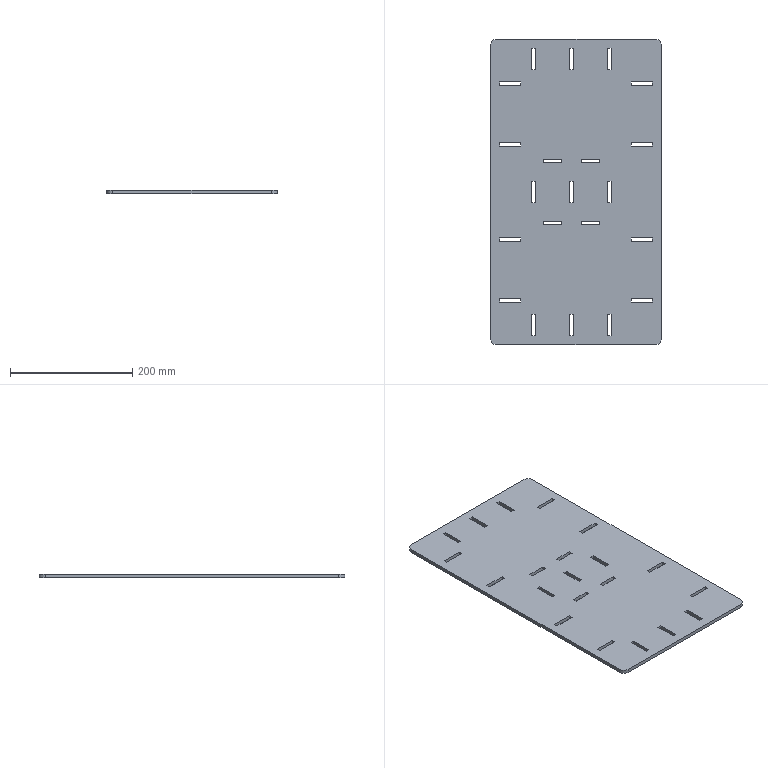Part | SolidWorks | features FlatPattern 1, SMBaseFlange 1, SheetMetal 1 | 1 solid | 94 faces | box 280 x 500 x 6 mm | volume 813715 mm3 | plane 90 | cylinder 4 | commonest cylinder face diameters 20.573 x4